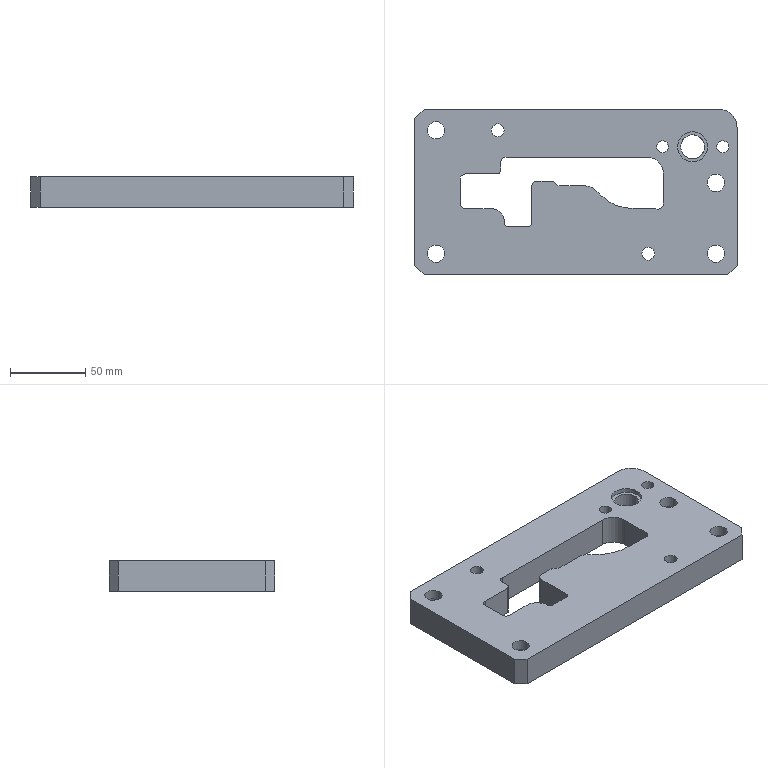Part | STEP file | lll_id218_x_t | 1 solid | 56 faces | box 214 x 110 x 20 mm | volume 369849 mm3 | cylinder 30 | plane 26 | commonest cylinder face diameters 7 x6 5 x4 11.509 x4 18.007 x4 8 x2 8.505 x2